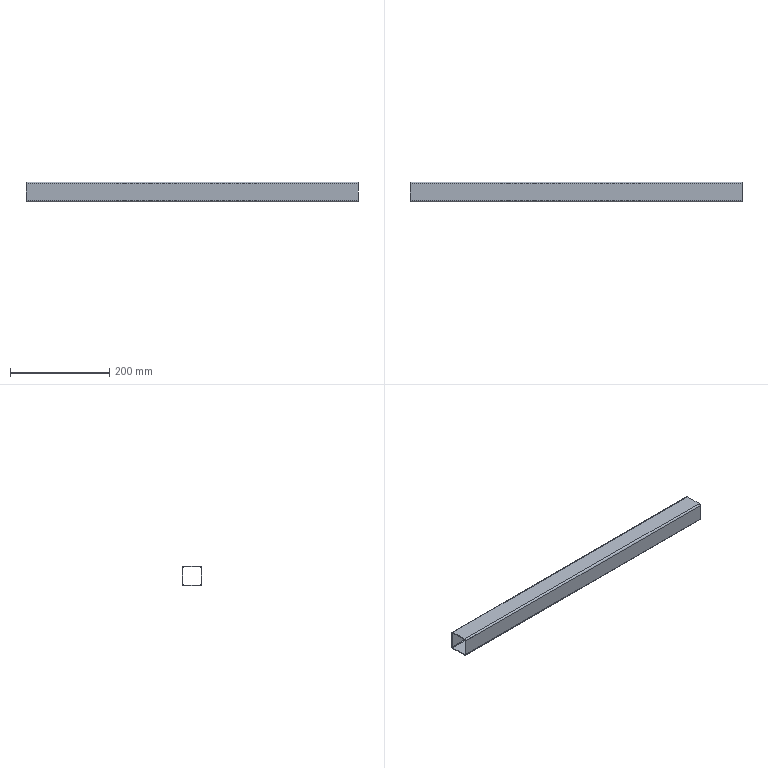Part | SolidWorks | features BaseBody 1 | 1 solid | 18 faces | box 670 x 40 x 40 mm | volume 174108 mm3 | plane 10 | cylinder 8 | commonest cylinder face diameters 3.5 x4 7 x4
STEP:
#1=CARTESIAN_POINT('',(-335.,20.,16.5));
#2=VERTEX_POINT('',#1);
#3=CARTESIAN_POINT('',(-335.,16.5,20.));
#4=VERTEX_POINT('',#3);
#5=CARTESIAN_POINT('',(-335.,16.5,16.5));
#6=DIRECTION('',(1.,0.,0.));
#7=DIRECTION('',(0.,0.,-1.));
#8=AXIS2_PLACEMENT_3D('',#5,#6,#7);
#9=CIRCLE('',#8,3.5);
#10=EDGE_CURVE('',#2,#4,#9,.T.);
#11=ORIENTED_EDGE('',*,*,#10,.T.);
#12=CARTESIAN_POINT('',(335.,16.5,20.));
#13=VERTEX_POINT('',#12);
#14=CARTESIAN_POINT('',(335.,16.5,20.));
#15=DIRECTION('',(-1.,0.,0.));
#16=VECTOR('',#15,1000.);
#17=LINE('',#14,#16);
#18=EDGE_CURVE('',#13,#4,#17,.T.);
#19=ORIENTED_EDGE('',*,*,#18,.F.);
#20=CARTESIAN_POINT('',(335.,20.,16.5));
#21=VERTEX_POINT('',#20);
#22=CARTESIAN_POINT('',(335.,16.5,16.5));
#23=DIRECTION('',(1.,0.,0.));
#24=DIRECTION('',(0.,0.,-1.));
#25=AXIS2_PLACEMENT_3D('',#22,#23,#24);
#26=CIRCLE('',#25,3.5);
#27=EDGE_CURVE('',#21,#13,#26,.T.);
#28=ORIENTED_EDGE('',*,*,#27,.F.);
#29=CARTESIAN_POINT('',(335.,20.,16.5));
#30=DIRECTION('',(-1.,0.,0.));
#31=VECTOR('',#30,1000.);
#32=LINE('',#29,#31);
#33=EDGE_CURVE('',#21,#2,#32,.T.);
#34=ORIENTED_EDGE('',*,*,#33,.T.);
#35=EDGE_LOOP('',(#11,#19,#28,#34));
#36=FACE_OUTER_BOUND('',#35,.T.);
#37=CARTESIAN_POINT('',(335.,16.5,16.5));
#38=DIRECTION('',(-1.,0.,0.));
#39=DIRECTION('',(0.,0.,1.));
#40=AXIS2_PLACEMENT_3D('',#37,#38,#39);
#41=CYLINDRICAL_SURFACE('',#40,3.5);
#42=ADVANCED_FACE('',(#36),#41,.T.);
#43=CARTESIAN_POINT('',(-335.,-16.5,20.));
#44=VERTEX_POINT('',#43);
#45=CARTESIAN_POINT('',(-335.,16.5,20.));
#46=DIRECTION('',(0.,-1.,0.));
#47=VECTOR('',#46,1000.);
#48=LINE('',#45,#47);
#49=EDGE_CURVE('',#4,#44,#48,.T.);
#50=ORIENTED_EDGE('',*,*,#49,.T.);
#51=CARTESIAN_POINT('',(335.,-16.5,20.));
#52=VERTEX_POINT('',#51);
#53=CARTESIAN_POINT('',(335.,-16.5,20.));
#54=DIRECTION('',(-1.,0.,0.));
#55=VECTOR('',#54,1000.);
#56=LINE('',#53,#55);
#57=EDGE_CURVE('',#52,#44,#56,.T.);
#58=ORIENTED_EDGE('',*,*,#57,.F.);
#59=CARTESIAN_POINT('',(335.,16.5,20.));
#60=DIRECTION('',(0.,-1.,0.));
#61=VECTOR('',#60,1000.);
#62=LINE('',#59,#61);
#63=EDGE_CURVE('',#13,#52,#62,.T.);
#64=ORIENTED_EDGE('',*,*,#63,.F.);
#65=ORIENTED_EDGE('',*,*,#18,.T.);
#66=EDGE_LOOP('',(#50,#58,#64,#65));
#67=FACE_OUTER_BOUND('',#66,.T.);
#68=CARTESIAN_POINT('',(335.,16.5,20.));
#69=DIRECTION('',(0.,0.,-1.));
#70=DIRECTION('',(-1.,0.,0.));
#71=AXIS2_PLACEMENT_3D('',#68,#69,#70);
#72=PLANE('',#71);
#73=ADVANCED_FACE('',(#67),#72,.F.);
#74=CARTESIAN_POINT('',(-335.,-20.,16.5));
#75=VERTEX_POINT('',#74);
#76=CARTESIAN_POINT('',(-335.,-16.5,16.5));
#77=DIRECTION('',(1.,0.,0.));
#78=DIRECTION('',(0.,0.,-1.));
#79=AXIS2_PLACEMENT_3D('',#76,#77,#78);
#80=CIRCLE('',#79,3.5);
#81=EDGE_CURVE('',#44,#75,#80,.T.);
#82=ORIENTED_EDGE('',*,*,#81,.T.);
#83=CARTESIAN_POINT('',(335.,-20.,16.5));
#84=VERTEX_POINT('',#83);
#85=CARTESIAN_POINT('',(335.,-20.,16.5));
#86=DIRECTION('',(-1.,0.,0.));
#87=VECTOR('',#86,1000.);
#88=LINE('',#85,#87);
#89=EDGE_CURVE('',#84,#75,#88,.T.);
#90=ORIENTED_EDGE('',*,*,#89,.F.);
#91=CARTESIAN_POINT('',(335.,-16.5,16.5));
#92=DIRECTION('',(1.,0.,0.));
#93=DIRECTION('',(0.,0.,-1.));
#94=AXIS2_PLACEMENT_3D('',#91,#92,#93);
#95=CIRCLE('',#94,3.5);
#96=EDGE_CURVE('',#52,#84,#95,.T.);
#97=ORIENTED_EDGE('',*,*,#96,.F.);
#98=ORIENTED_EDGE('',*,*,#57,.T.);
#99=EDGE_LOOP('',(#82,#90,#97,#98));
#100=FACE_OUTER_BOUND('',#99,.T.);
#101=CARTESIAN_POINT('',(335.,-16.5,16.5));
#102=DIRECTION('',(-1.,0.,0.));
#103=DIRECTION('',(0.,0.,1.));
#104=AXIS2_PLACEMENT_3D('',#101,#102,#103);
#105=CYLINDRICAL_SURFACE('',#104,3.5);
#106=ADVANCED_FACE('',(#100),#105,.T.);
#107=CARTESIAN_POINT('',(-335.,-20.,-16.5));
#108=VERTEX_POINT('',#107);
#109=CARTESIAN_POINT('',(-335.,-20.,-16.5));
#110=DIRECTION('',(0.,0.,-1.));
#111=VECTOR('',#110,1000.);
#112=LINE('',#109,#111);
#113=EDGE_CURVE('',#75,#108,#112,.T.);
#114=ORIENTED_EDGE('',*,*,#113,.T.);
#115=CARTESIAN_POINT('',(335.,-20.,-16.5));
#116=VERTEX_POINT('',#115);
#117=CARTESIAN_POINT('',(335.,-20.,-16.5));
#118=DIRECTION('',(-1.,0.,0.));
#119=VECTOR('',#118,1000.);
#120=LINE('',#117,#119);
#121=EDGE_CURVE('',#116,#108,#120,.T.);
#122=ORIENTED_EDGE('',*,*,#121,.F.);
#123=CARTESIAN_POINT('',(335.,-20.,-16.5));
#124=DIRECTION('',(0.,0.,-1.));
#125=VECTOR('',#124,1000.);
#126=LINE('',#123,#125);
#127=EDGE_CURVE('',#84,#116,#126,.T.);
#128=ORIENTED_EDGE('',*,*,#127,.F.);
#129=ORIENTED_EDGE('',*,*,#89,.T.);
#130=EDGE_LOOP('',(#114,#122,#128,#129));
#131=FACE_OUTER_BOUND('',#130,.T.);
#132=CARTESIAN_POINT('',(335.,-20.,-16.5));
#133=DIRECTION('',(0.,1.,0.));
#134=DIRECTION('',(0.,0.,1.));
#135=AXIS2_PLACEMENT_3D('',#132,#133,#134);
#136=PLANE('',#135);
#137=ADVANCED_FACE('',(#131),#136,.F.);
#138=CARTESIAN_POINT('',(-335.,-16.5,-20.));
#139=VERTEX_POINT('',#138);
#140=CARTESIAN_POINT('',(-335.,-16.5,-16.5));
#141=DIRECTION('',(1.,0.,0.));
#142=DIRECTION('',(0.,0.,-1.));
#143=AXIS2_PLACEMENT_3D('',#140,#141,#142);
#144=CIRCLE('',#143,3.5);
#145=EDGE_CURVE('',#108,#139,#144,.T.);
#146=ORIENTED_EDGE('',*,*,#145,.T.);
#147=CARTESIAN_POINT('',(335.,-16.5,-20.));
#148=VERTEX_POINT('',#147);
#149=CARTESIAN_POINT('',(335.,-16.5,-20.));
#150=DIRECTION('',(-1.,0.,0.));
#151=VECTOR('',#150,1000.);
#152=LINE('',#149,#151);
#153=EDGE_CURVE('',#148,#139,#152,.T.);
#154=ORIENTED_EDGE('',*,*,#153,.F.);
#155=CARTESIAN_POINT('',(335.,-16.5,-16.5));
#156=DIRECTION('',(1.,0.,0.));
#157=DIRECTION('',(0.,0.,-1.));
#158=AXIS2_PLACEMENT_3D('',#155,#156,#157);
#159=CIRCLE('',#158,3.5);
#160=EDGE_CURVE('',#116,#148,#159,.T.);
#161=ORIENTED_EDGE('',*,*,#160,.F.);
#162=ORIENTED_EDGE('',*,*,#121,.T.);
#163=EDGE_LOOP('',(#146,#154,#161,#162));
#164=FACE_OUTER_BOUND('',#163,.T.);
#165=CARTESIAN_POINT('',(335.,-16.5,-16.5));
#166=DIRECTION('',(-1.,0.,0.));
#167=DIRECTION('',(0.,0.,1.));
#168=AXIS2_PLACEMENT_3D('',#165,#166,#167);
#169=CYLINDRICAL_SURFACE('',#168,3.5);
#170=ADVANCED_FACE('',(#164),#169,.T.);
#171=CARTESIAN_POINT('',(-335.,16.5,-20.));
#172=VERTEX_POINT('',#171);
#173=CARTESIAN_POINT('',(-335.,-16.5,-20.));
#174=DIRECTION('',(0.,1.,0.));
#175=VECTOR('',#174,1000.);
#176=LINE('',#173,#175);
#177=EDGE_CURVE('',#139,#172,#176,.T.);
#178=ORIENTED_EDGE('',*,*,#177,.T.);
#179=CARTESIAN_POINT('',(335.,16.5,-20.));
#180=VERTEX_POINT('',#179);
#181=CARTESIAN_POINT('',(335.,16.5,-20.));
#182=DIRECTION('',(-1.,0.,0.));
#183=VECTOR('',#182,1000.);
#184=LINE('',#181,#183);
#185=EDGE_CURVE('',#180,#172,#184,.T.);
#186=ORIENTED_EDGE('',*,*,#185,.F.);
#187=CARTESIAN_POINT('',(335.,-16.5,-20.));
#188=DIRECTION('',(0.,1.,0.));
#189=VECTOR('',#188,1000.);
#190=LINE('',#187,#189);
#191=EDGE_CURVE('',#148,#180,#190,.T.);
#192=ORIENTED_EDGE('',*,*,#191,.F.);
#193=ORIENTED_EDGE('',*,*,#153,.T.);
#194=EDGE_LOOP('',(#178,#186,#192,#193));
#195=FACE_OUTER_BOUND('',#194,.T.);
#196=CARTESIAN_POINT('',(335.,-16.5,-20.));
#197=DIRECTION('',(0.,0.,1.));
#198=DIRECTION('',(1.,0.,0.));
#199=AXIS2_PLACEMENT_3D('',#196,#197,#198);
#200=PLANE('',#199);
#201=ADVANCED_FACE('',(#195),#200,.F.);
#202=CARTESIAN_POINT('',(-335.,20.,-16.5));
#203=VERTEX_POINT('',#202);
#204=CARTESIAN_POINT('',(-335.,16.5,-16.5));
#205=DIRECTION('',(1.,0.,0.));
#206=DIRECTION('',(0.,0.,-1.));
#207=AXIS2_PLACEMENT_3D('',#204,#205,#206);
#208=CIRCLE('',#207,3.5);
#209=EDGE_CURVE('',#172,#203,#208,.T.);
#210=ORIENTED_EDGE('',*,*,#209,.T.);
#211=CARTESIAN_POINT('',(335.,20.,-16.5));
#212=VERTEX_POINT('',#211);
#213=CARTESIAN_POINT('',(335.,20.,-16.5));
#214=DIRECTION('',(-1.,0.,0.));
#215=VECTOR('',#214,1000.);
#216=LINE('',#213,#215);
#217=EDGE_CURVE('',#212,#203,#216,.T.);
#218=ORIENTED_EDGE('',*,*,#217,.F.);
#219=CARTESIAN_POINT('',(335.,16.5,-16.5));
#220=DIRECTION('',(1.,0.,0.));
#221=DIRECTION('',(0.,0.,-1.));
#222=AXIS2_PLACEMENT_3D('',#219,#220,#221);
#223=CIRCLE('',#222,3.5);
#224=EDGE_CURVE('',#180,#212,#223,.T.);
#225=ORIENTED_EDGE('',*,*,#224,.F.);
#226=ORIENTED_EDGE('',*,*,#185,.T.);
#227=EDGE_LOOP('',(#210,#218,#225,#226));
#228=FACE_OUTER_BOUND('',#227,.T.);
#229=CARTESIAN_POINT('',(335.,16.5,-16.5));
#230=DIRECTION('',(-1.,0.,0.));
#231=DIRECTION('',(0.,0.,1.));
#232=AXIS2_PLACEMENT_3D('',#229,#230,#231);
#233=CYLINDRICAL_SURFACE('',#232,3.5);
#234=ADVANCED_FACE('',(#228),#233,.T.);
#235=CARTESIAN_POINT('',(-335.,-16.5,18.25));
#236=VERTEX_POINT('',#235);
#237=CARTESIAN_POINT('',(-335.,-18.25,16.5));
#238=VERTEX_POINT('',#237);
#239=CARTESIAN_POINT('',(-335.,-16.5,16.5));
#240=DIRECTION('',(1.,0.,0.));
#241=DIRECTION('',(0.,0.,-1.));
#242=AXIS2_PLACEMENT_3D('',#239,#240,#241);
#243=CIRCLE('',#242,1.75);
#244=EDGE_CURVE('',#236,#238,#243,.T.);
#245=ORIENTED_EDGE('',*,*,#244,.F.);
#246=CARTESIAN_POINT('',(335.,-16.5,18.25));
#247=VERTEX_POINT('',#246);
#248=CARTESIAN_POINT('',(335.,-16.5,18.25));
#249=DIRECTION('',(-1.,0.,0.));
#250=VECTOR('',#249,1000.);
#251=LINE('',#248,#250);
#252=EDGE_CURVE('',#247,#236,#251,.T.);
#253=ORIENTED_EDGE('',*,*,#252,.F.);
#254=CARTESIAN_POINT('',(335.,-18.25,16.5));
#255=VERTEX_POINT('',#254);
#256=CARTESIAN_POINT('',(335.,-16.5,16.5));
#257=DIRECTION('',(1.,0.,0.));
#258=DIRECTION('',(0.,0.,-1.));
#259=AXIS2_PLACEMENT_3D('',#256,#257,#258);
#260=CIRCLE('',#259,1.75);
#261=EDGE_CURVE('',#247,#255,#260,.T.);
#262=ORIENTED_EDGE('',*,*,#261,.T.);
#263=CARTESIAN_POINT('',(335.,-18.25,16.5));
#264=DIRECTION('',(-1.,0.,0.));
#265=VECTOR('',#264,1000.);
#266=LINE('',#263,#265);
#267=EDGE_CURVE('',#255,#238,#266,.T.);
#268=ORIENTED_EDGE('',*,*,#267,.T.);
#269=EDGE_LOOP('',(#245,#253,#262,#268));
#270=FACE_OUTER_BOUND('',#269,.T.);
#271=CARTESIAN_POINT('',(335.,-16.5,16.5));
#272=DIRECTION('',(-1.,0.,0.));
#273=DIRECTION('',(0.,0.,1.));
#274=AXIS2_PLACEMENT_3D('',#271,#272,#273);
#275=CYLINDRICAL_SURFACE('',#274,1.75);
#276=ADVANCED_FACE('',(#270),#275,.F.);
#277=CARTESIAN_POINT('',(-335.,16.5,18.25));
#278=VERTEX_POINT('',#277);
#279=CARTESIAN_POINT('',(-335.,16.5,18.25));
#280=DIRECTION('',(0.,-1.,0.));
#281=VECTOR('',#280,1000.);
#282=LINE('',#279,#281);
#283=EDGE_CURVE('',#278,#236,#282,.T.);
#284=ORIENTED_EDGE('',*,*,#283,.F.);
#285=CARTESIAN_POINT('',(335.,16.5,18.25));
#286=VERTEX_POINT('',#285);
#287=CARTESIAN_POINT('',(335.,16.5,18.25));
#288=DIRECTION('',(-1.,0.,0.));
#289=VECTOR('',#288,1000.);
#290=LINE('',#287,#289);
#291=EDGE_CURVE('',#286,#278,#290,.T.);
#292=ORIENTED_EDGE('',*,*,#291,.F.);
#293=CARTESIAN_POINT('',(335.,16.5,18.25));
#294=DIRECTION('',(0.,-1.,0.));
#295=VECTOR('',#294,1000.);
#296=LINE('',#293,#295);
#297=EDGE_CURVE('',#286,#247,#296,.T.);
#298=ORIENTED_EDGE('',*,*,#297,.T.);
#299=ORIENTED_EDGE('',*,*,#252,.T.);
#300=EDGE_LOOP('',(#284,#292,#298,#299));
#301=FACE_OUTER_BOUND('',#300,.T.);
#302=CARTESIAN_POINT('',(335.,16.5,18.25));
#303=DIRECTION('',(0.,0.,-1.));
#304=DIRECTION('',(-1.,0.,0.));
#305=AXIS2_PLACEMENT_3D('',#302,#303,#304);
#306=PLANE('',#305);
#307=ADVANCED_FACE('',(#301),#306,.T.);
#308=CARTESIAN_POINT('',(-335.,18.25,16.5));
#309=VERTEX_POINT('',#308);
#310=CARTESIAN_POINT('',(-335.,16.5,16.5));
#311=DIRECTION('',(1.,0.,0.));
#312=DIRECTION('',(0.,0.,-1.));
#313=AXIS2_PLACEMENT_3D('',#310,#311,#312);
#314=CIRCLE('',#313,1.75);
#315=EDGE_CURVE('',#309,#278,#314,.T.);
#316=ORIENTED_EDGE('',*,*,#315,.F.);
#317=CARTESIAN_POINT('',(335.,18.25,16.5));
#318=VERTEX_POINT('',#317);
#319=CARTESIAN_POINT('',(335.,18.25,16.5));
#320=DIRECTION('',(-1.,0.,0.));
#321=VECTOR('',#320,1000.);
#322=LINE('',#319,#321);
#323=EDGE_CURVE('',#318,#309,#322,.T.);
#324=ORIENTED_EDGE('',*,*,#323,.F.);
#325=CARTESIAN_POINT('',(335.,16.5,16.5));
#326=DIRECTION('',(1.,0.,0.));
#327=DIRECTION('',(0.,0.,-1.));
#328=AXIS2_PLACEMENT_3D('',#325,#326,#327);
#329=CIRCLE('',#328,1.75);
#330=EDGE_CURVE('',#318,#286,#329,.T.);
#331=ORIENTED_EDGE('',*,*,#330,.T.);
#332=ORIENTED_EDGE('',*,*,#291,.T.);
#333=EDGE_LOOP('',(#316,#324,#331,#332));
#334=FACE_OUTER_BOUND('',#333,.T.);
#335=CARTESIAN_POINT('',(335.,16.5,16.5));
#336=DIRECTION('',(-1.,0.,0.));
#337=DIRECTION('',(0.,0.,1.));
#338=AXIS2_PLACEMENT_3D('',#335,#336,#337);
#339=CYLINDRICAL_SURFACE('',#338,1.75);
#340=ADVANCED_FACE('',(#334),#339,.F.);
#341=CARTESIAN_POINT('',(-335.,18.25,-16.5));
#342=VERTEX_POINT('',#341);
#343=CARTESIAN_POINT('',(-335.,18.25,16.5));
#344=DIRECTION('',(0.,0.,1.));
#345=VECTOR('',#344,1000.);
#346=LINE('',#343,#345);
#347=EDGE_CURVE('',#342,#309,#346,.T.);
#348=ORIENTED_EDGE('',*,*,#347,.F.);
#349=CARTESIAN_POINT('',(335.,18.25,-16.5));
#350=VERTEX_POINT('',#349);
#351=CARTESIAN_POINT('',(335.,18.25,-16.5));
#352=DIRECTION('',(-1.,0.,0.));
#353=VECTOR('',#352,1000.);
#354=LINE('',#351,#353);
#355=EDGE_CURVE('',#350,#342,#354,.T.);
#356=ORIENTED_EDGE('',*,*,#355,.F.);
#357=CARTESIAN_POINT('',(335.,18.25,16.5));
#358=DIRECTION('',(0.,0.,1.));
#359=VECTOR('',#358,1000.);
#360=LINE('',#357,#359);
#361=EDGE_CURVE('',#350,#318,#360,.T.);
#362=ORIENTED_EDGE('',*,*,#361,.T.);
#363=ORIENTED_EDGE('',*,*,#323,.T.);
#364=EDGE_LOOP('',(#348,#356,#362,#363));
#365=FACE_OUTER_BOUND('',#364,.T.);
#366=CARTESIAN_POINT('',(335.,18.25,16.5));
#367=DIRECTION('',(0.,-1.,0.));
#368=DIRECTION('',(0.,0.,-1.));
#369=AXIS2_PLACEMENT_3D('',#366,#367,#368);
#370=PLANE('',#369);
#371=ADVANCED_FACE('',(#365),#370,.T.);
#372=CARTESIAN_POINT('',(-335.,16.5,-18.25));
#373=VERTEX_POINT('',#372);
#374=CARTESIAN_POINT('',(-335.,16.5,-16.5));
#375=DIRECTION('',(1.,0.,0.));
#376=DIRECTION('',(0.,0.,-1.));
#377=AXIS2_PLACEMENT_3D('',#374,#375,#376);
#378=CIRCLE('',#377,1.75);
#379=EDGE_CURVE('',#373,#342,#378,.T.);
#380=ORIENTED_EDGE('',*,*,#379,.F.);
#381=CARTESIAN_POINT('',(335.,16.5,-18.25));
#382=VERTEX_POINT('',#381);
#383=CARTESIAN_POINT('',(335.,16.5,-18.25));
#384=DIRECTION('',(-1.,0.,0.));
#385=VECTOR('',#384,1000.);
#386=LINE('',#383,#385);
#387=EDGE_CURVE('',#382,#373,#386,.T.);
#388=ORIENTED_EDGE('',*,*,#387,.F.);
#389=CARTESIAN_POINT('',(335.,16.5,-16.5));
#390=DIRECTION('',(1.,0.,0.));
#391=DIRECTION('',(0.,0.,-1.));
#392=AXIS2_PLACEMENT_3D('',#389,#390,#391);
#393=CIRCLE('',#392,1.75);
#394=EDGE_CURVE('',#382,#350,#393,.T.);
#395=ORIENTED_EDGE('',*,*,#394,.T.);
#396=ORIENTED_EDGE('',*,*,#355,.T.);
#397=EDGE_LOOP('',(#380,#388,#395,#396));
#398=FACE_OUTER_BOUND('',#397,.T.);
#399=CARTESIAN_POINT('',(335.,16.5,-16.5));
#400=DIRECTION('',(-1.,0.,0.));
#401=DIRECTION('',(0.,0.,1.));
#402=AXIS2_PLACEMENT_3D('',#399,#400,#401);
#403=CYLINDRICAL_SURFACE('',#402,1.75);
#404=ADVANCED_FACE('',(#398),#403,.F.);
#405=CARTESIAN_POINT('',(-335.,-16.5,-18.25));
#406=VERTEX_POINT('',#405);
#407=CARTESIAN_POINT('',(-335.,-16.5,-18.25));
#408=DIRECTION('',(0.,1.,0.));
#409=VECTOR('',#408,1000.);
#410=LINE('',#407,#409);
#411=EDGE_CURVE('',#406,#373,#410,.T.);
#412=ORIENTED_EDGE('',*,*,#411,.F.);
#413=CARTESIAN_POINT('',(335.,-16.5,-18.25));
#414=VERTEX_POINT('',#413);
#415=CARTESIAN_POINT('',(335.,-16.5,-18.25));
#416=DIRECTION('',(-1.,0.,0.));
#417=VECTOR('',#416,1000.);
#418=LINE('',#415,#417);
#419=EDGE_CURVE('',#414,#406,#418,.T.);
#420=ORIENTED_EDGE('',*,*,#419,.F.);
#421=CARTESIAN_POINT('',(335.,-16.5,-18.25));
#422=DIRECTION('',(0.,1.,0.));
#423=VECTOR('',#422,1000.);
#424=LINE('',#421,#423);
#425=EDGE_CURVE('',#414,#382,#424,.T.);
#426=ORIENTED_EDGE('',*,*,#425,.T.);
#427=ORIENTED_EDGE('',*,*,#387,.T.);
#428=EDGE_LOOP('',(#412,#420,#426,#427));
#429=FACE_OUTER_BOUND('',#428,.T.);
#430=CARTESIAN_POINT('',(335.,-16.5,-18.25));
#431=DIRECTION('',(0.,0.,1.));
#432=DIRECTION('',(1.,0.,0.));
#433=AXIS2_PLACEMENT_3D('',#430,#431,#432);
#434=PLANE('',#433);
#435=ADVANCED_FACE('',(#429),#434,.T.);
#436=CARTESIAN_POINT('',(-335.,-18.25,-16.5));
#437=VERTEX_POINT('',#436);
#438=CARTESIAN_POINT('',(-335.,-16.5,-16.5));
#439=DIRECTION('',(1.,0.,0.));
#440=DIRECTION('',(0.,0.,-1.));
#441=AXIS2_PLACEMENT_3D('',#438,#439,#440);
#442=CIRCLE('',#441,1.75);
#443=EDGE_CURVE('',#437,#406,#442,.T.);
#444=ORIENTED_EDGE('',*,*,#443,.F.);
#445=CARTESIAN_POINT('',(335.,-18.25,-16.5));
#446=VERTEX_POINT('',#445);
#447=CARTESIAN_POINT('',(335.,-18.25,-16.5));
#448=DIRECTION('',(-1.,0.,0.));
#449=VECTOR('',#448,1000.);
#450=LINE('',#447,#449);
#451=EDGE_CURVE('',#446,#437,#450,.T.);
#452=ORIENTED_EDGE('',*,*,#451,.F.);
#453=CARTESIAN_POINT('',(335.,-16.5,-16.5));
#454=DIRECTION('',(1.,0.,0.));
#455=DIRECTION('',(0.,0.,-1.));
#456=AXIS2_PLACEMENT_3D('',#453,#454,#455);
#457=CIRCLE('',#456,1.75);
#458=EDGE_CURVE('',#446,#414,#457,.T.);
#459=ORIENTED_EDGE('',*,*,#458,.T.);
#460=ORIENTED_EDGE('',*,*,#419,.T.);
#461=EDGE_LOOP('',(#444,#452,#459,#460));
#462=FACE_OUTER_BOUND('',#461,.T.);
#463=CARTESIAN_POINT('',(335.,-16.5,-16.5));
#464=DIRECTION('',(-1.,0.,0.));
#465=DIRECTION('',(0.,0.,1.));
#466=AXIS2_PLACEMENT_3D('',#463,#464,#465);
#467=CYLINDRICAL_SURFACE('',#466,1.75);
#468=ADVANCED_FACE('',(#462),#467,.F.);
#469=CARTESIAN_POINT('',(-335.,-18.25,-16.5));
#470=DIRECTION('',(0.,0.,-1.));
#471=VECTOR('',#470,1000.);
#472=LINE('',#469,#471);
#473=EDGE_CURVE('',#238,#437,#472,.T.);
#474=ORIENTED_EDGE('',*,*,#473,.F.);
#475=ORIENTED_EDGE('',*,*,#267,.F.);
#476=CARTESIAN_POINT('',(335.,-18.25,-16.5));
#477=DIRECTION('',(0.,0.,-1.));
#478=VECTOR('',#477,1000.);
#479=LINE('',#476,#478);
#480=EDGE_CURVE('',#255,#446,#479,.T.);
#481=ORIENTED_EDGE('',*,*,#480,.T.);
#482=ORIENTED_EDGE('',*,*,#451,.T.);
#483=EDGE_LOOP('',(#474,#475,#481,#482));
#484=FACE_OUTER_BOUND('',#483,.T.);
#485=CARTESIAN_POINT('',(335.,-18.25,-16.5));
#486=DIRECTION('',(0.,1.,0.));
#487=DIRECTION('',(0.,0.,1.));
#488=AXIS2_PLACEMENT_3D('',#485,#486,#487);
#489=PLANE('',#488);
#490=ADVANCED_FACE('',(#484),#489,.T.);
#491=CARTESIAN_POINT('',(-335.,20.,16.5));
#492=DIRECTION('',(0.,0.,1.));
#493=VECTOR('',#492,1000.);
#494=LINE('',#491,#493);
#495=EDGE_CURVE('',#203,#2,#494,.T.);
#496=ORIENTED_EDGE('',*,*,#495,.T.);
#497=ORIENTED_EDGE('',*,*,#33,.F.);
#498=CARTESIAN_POINT('',(335.,20.,16.5));
#499=DIRECTION('',(0.,0.,1.));
#500=VECTOR('',#499,1000.);
#501=LINE('',#498,#500);
#502=EDGE_CURVE('',#212,#21,#501,.T.);
#503=ORIENTED_EDGE('',*,*,#502,.F.);
#504=ORIENTED_EDGE('',*,*,#217,.T.);
#505=EDGE_LOOP('',(#496,#497,#503,#504));
#506=FACE_OUTER_BOUND('',#505,.T.);
#507=CARTESIAN_POINT('',(335.,20.,16.5));
#508=DIRECTION('',(0.,-1.,0.));
#509=DIRECTION('',(0.,0.,-1.));
#510=AXIS2_PLACEMENT_3D('',#507,#508,#509);
#511=PLANE('',#510);
#512=ADVANCED_FACE('',(#506),#511,.F.);
#513=ORIENTED_EDGE('',*,*,#261,.F.);
#514=ORIENTED_EDGE('',*,*,#297,.F.);
#515=ORIENTED_EDGE('',*,*,#330,.F.);
#516=ORIENTED_EDGE('',*,*,#361,.F.);
#517=ORIENTED_EDGE('',*,*,#394,.F.);
#518=ORIENTED_EDGE('',*,*,#425,.F.);
#519=ORIENTED_EDGE('',*,*,#458,.F.);
#520=ORIENTED_EDGE('',*,*,#480,.F.);
#521=EDGE_LOOP('',(#513,#514,#515,#516,#517,#518,#519,#520));
#522=FACE_BOUND('',#521,.T.);
#523=ORIENTED_EDGE('',*,*,#27,.T.);
#524=ORIENTED_EDGE('',*,*,#63,.T.);
#525=ORIENTED_EDGE('',*,*,#96,.T.);
#526=ORIENTED_EDGE('',*,*,#127,.T.);
#527=ORIENTED_EDGE('',*,*,#160,.T.);
#528=ORIENTED_EDGE('',*,*,#191,.T.);
#529=ORIENTED_EDGE('',*,*,#224,.T.);
#530=ORIENTED_EDGE('',*,*,#502,.T.);
#531=EDGE_LOOP('',(#523,#524,#525,#526,#527,#528,#529,#530));
#532=FACE_OUTER_BOUND('',#531,.T.);
#533=CARTESIAN_POINT('',(335.,16.5,16.5));
#534=DIRECTION('',(1.,0.,0.));
#535=DIRECTION('',(0.,0.,-1.));
#536=AXIS2_PLACEMENT_3D('',#533,#534,#535);
#537=PLANE('',#536);
#538=ADVANCED_FACE('',(#522,#532),#537,.T.);
#539=ORIENTED_EDGE('',*,*,#244,.T.);
#540=ORIENTED_EDGE('',*,*,#473,.T.);
#541=ORIENTED_EDGE('',*,*,#443,.T.);
#542=ORIENTED_EDGE('',*,*,#411,.T.);
#543=ORIENTED_EDGE('',*,*,#379,.T.);
#544=ORIENTED_EDGE('',*,*,#347,.T.);
#545=ORIENTED_EDGE('',*,*,#315,.T.);
#546=ORIENTED_EDGE('',*,*,#283,.T.);
#547=EDGE_LOOP('',(#539,#540,#541,#542,#543,#544,#545,#546));
#548=FACE_BOUND('',#547,.T.);
#549=ORIENTED_EDGE('',*,*,#10,.F.);
#550=ORIENTED_EDGE('',*,*,#495,.F.);
#551=ORIENTED_EDGE('',*,*,#209,.F.);
#552=ORIENTED_EDGE('',*,*,#177,.F.);
#553=ORIENTED_EDGE('',*,*,#145,.F.);
#554=ORIENTED_EDGE('',*,*,#113,.F.);
#555=ORIENTED_EDGE('',*,*,#81,.F.);
#556=ORIENTED_EDGE('',*,*,#49,.F.);
#557=EDGE_LOOP('',(#549,#550,#551,#552,#553,#554,#555,#556));
#558=FACE_OUTER_BOUND('',#557,.T.);
#559=CARTESIAN_POINT('',(-335.,16.5,16.5));
#560=DIRECTION('',(1.,0.,0.));
#561=DIRECTION('',(0.,0.,-1.));
#562=AXIS2_PLACEMENT_3D('',#559,#560,#561);
#563=PLANE('',#562);
#564=ADVANCED_FACE('',(#548,#558),#563,.F.);
#565=CLOSED_SHELL('',(#42,#73,#106,#137,#170,#201,#234,#276,#307,#340,#371,#404,#435,#468,#490,#512,#538,#564));
#566=MANIFOLD_SOLID_BREP('',#565);
#567=CARTESIAN_POINT('',(0.,0.,0.));
#568=DIRECTION('',(0.,0.,1.));
#569=DIRECTION('',(1.,0.,0.));
#570=AXIS2_PLACEMENT_3D('',#567,#568,#569);
#571=(LENGTH_UNIT()NAMED_UNIT(*)SI_UNIT(.MILLI.,.METRE.));
#572=UNCERTAINTY_MEASURE_WITH_UNIT(LENGTH_MEASURE(0.00001),#571,'','');
#573=(NAMED_UNIT(*)PLANE_ANGLE_UNIT()SI_UNIT($,.RADIAN.));
#574=(NAMED_UNIT(*)SI_UNIT($,.STERADIAN.)SOLID_ANGLE_UNIT());
#575=(GEOMETRIC_REPRESENTATION_CONTEXT(3)GLOBAL_UNCERTAINTY_ASSIGNED_CONTEXT((#572))GLOBAL_UNIT_ASSIGNED_CONTEXT((#571,#573,#574))REPRESENTATION_CONTEXT('',''));
#576=ADVANCED_BREP_SHAPE_REPRESENTATION('',(#566,#570),#575);